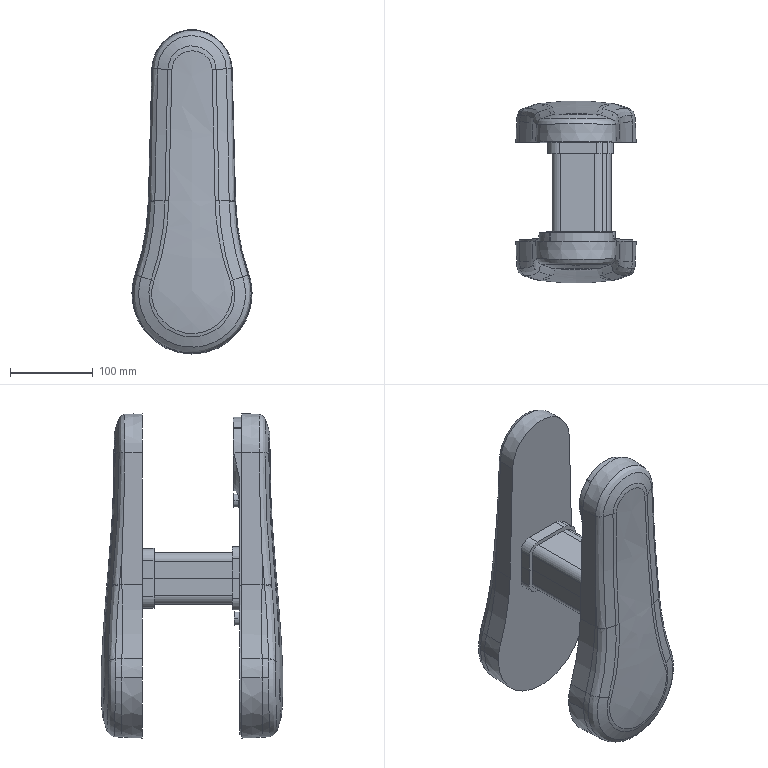Part | STEP file | ASND-0110-IRB120_3-58_IRC5_Link2_rev0 | 10 solids | 279 faces | box 144.86 x 219.43 x 390.86 mm | volume 3910323 mm3 | cylinder 89 | plane 72 | spline 54 | cone 35 | torus 29 | commonest cylinder face diameters 8 x24 28 x12 20 x8 3.3 x6 6.4 x6 7.134 x6